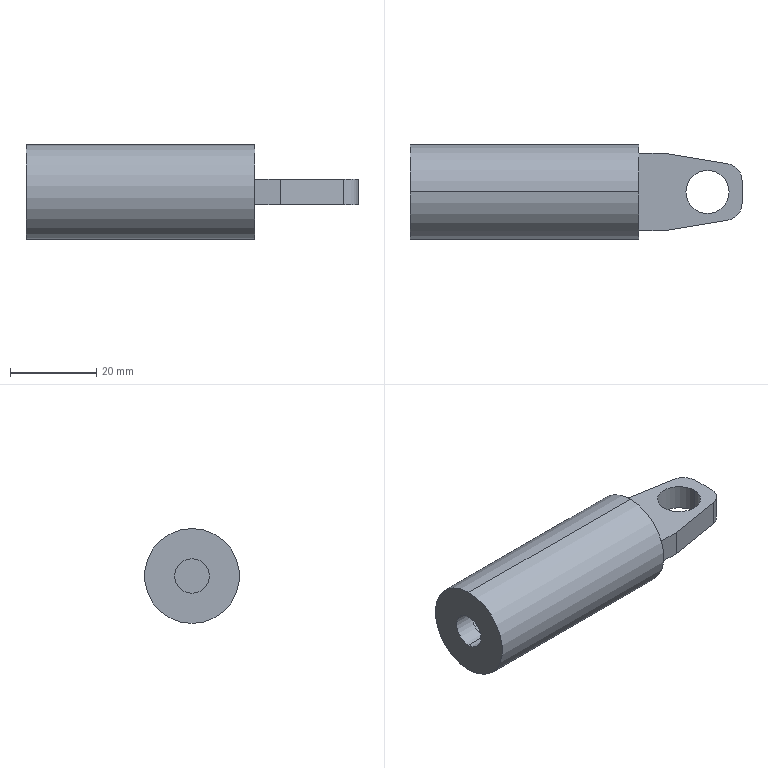Part | SolidWorks | features HoleWzd 2, Fillet 1, ICE 1, Revolution 1 | 1 solid | 21 faces | box 77 x 22 x 22 mm | volume 12617 mm3 | plane 11 | cylinder 10 | commonest cylinder face diameters 8 x4 10 x2 16 x2 22 x2
STEP:
#1=CARTESIAN_POINT('',(5.,0.,-4.));
#2=VERTEX_POINT('',#1);
#3=CARTESIAN_POINT('',(5.,0.,4.));
#4=VERTEX_POINT('',#3);
#5=CARTESIAN_POINT('',(5.,0.,0.));
#6=DIRECTION('',(-1.,0.,0.));
#7=DIRECTION('',(0.,0.,1.));
#8=AXIS2_PLACEMENT_3D('',#5,#6,#7);
#9=CIRCLE('',#8,4.);
#10=EDGE_CURVE('',#2,#4,#9,.T.);
#11=ORIENTED_EDGE('',*,*,#10,.F.);
#12=CARTESIAN_POINT('',(0.,0.,-4.));
#13=VERTEX_POINT('',#12);
#14=CARTESIAN_POINT('',(0.,0.,-4.));
#15=DIRECTION('',(-1.,0.,0.));
#16=VECTOR('',#15,1000.);
#17=LINE('',#14,#16);
#18=EDGE_CURVE('',#2,#13,#17,.T.);
#19=ORIENTED_EDGE('',*,*,#18,.T.);
#20=CARTESIAN_POINT('',(0.,0.,4.));
#21=VERTEX_POINT('',#20);
#22=CARTESIAN_POINT('',(0.,0.,0.));
#23=DIRECTION('',(-1.,0.,0.));
#24=DIRECTION('',(0.,0.,1.));
#25=AXIS2_PLACEMENT_3D('',#22,#23,#24);
#26=CIRCLE('',#25,4.);
#27=EDGE_CURVE('',#13,#21,#26,.T.);
#28=ORIENTED_EDGE('',*,*,#27,.T.);
#29=CARTESIAN_POINT('',(0.,0.,4.));
#30=DIRECTION('',(-1.,0.,0.));
#31=VECTOR('',#30,1000.);
#32=LINE('',#29,#31);
#33=EDGE_CURVE('',#4,#21,#32,.T.);
#34=ORIENTED_EDGE('',*,*,#33,.F.);
#35=EDGE_LOOP('',(#11,#19,#28,#34));
#36=FACE_OUTER_BOUND('',#35,.T.);
#37=CARTESIAN_POINT('',(0.,0.,0.));
#38=DIRECTION('',(-1.,0.,0.));
#39=DIRECTION('',(0.,0.,1.));
#40=AXIS2_PLACEMENT_3D('',#37,#38,#39);
#41=CYLINDRICAL_SURFACE('',#40,4.);
#42=ADVANCED_FACE('',(#36),#41,.F.);
#43=CARTESIAN_POINT('',(50.,0.,-8.));
#44=VERTEX_POINT('',#43);
#45=CARTESIAN_POINT('',(50.,0.,8.));
#46=VERTEX_POINT('',#45);
#47=CARTESIAN_POINT('',(50.,0.,0.));
#48=DIRECTION('',(-1.,0.,0.));
#49=DIRECTION('',(0.,0.,1.));
#50=AXIS2_PLACEMENT_3D('',#47,#48,#49);
#51=CIRCLE('',#50,8.);
#52=EDGE_CURVE('',#44,#46,#51,.T.);
#53=ORIENTED_EDGE('',*,*,#52,.F.);
#54=CARTESIAN_POINT('',(5.,0.,-8.));
#55=VERTEX_POINT('',#54);
#56=CARTESIAN_POINT('',(0.,0.,-8.));
#57=DIRECTION('',(-1.,0.,0.));
#58=VECTOR('',#57,1000.);
#59=LINE('',#56,#58);
#60=EDGE_CURVE('',#44,#55,#59,.T.);
#61=ORIENTED_EDGE('',*,*,#60,.T.);
#62=CARTESIAN_POINT('',(5.,0.,8.));
#63=VERTEX_POINT('',#62);
#64=CARTESIAN_POINT('',(5.,0.,0.));
#65=DIRECTION('',(-1.,0.,0.));
#66=DIRECTION('',(0.,0.,1.));
#67=AXIS2_PLACEMENT_3D('',#64,#65,#66);
#68=CIRCLE('',#67,8.);
#69=EDGE_CURVE('',#55,#63,#68,.T.);
#70=ORIENTED_EDGE('',*,*,#69,.T.);
#71=CARTESIAN_POINT('',(0.,0.,8.));
#72=DIRECTION('',(-1.,0.,0.));
#73=VECTOR('',#72,1000.);
#74=LINE('',#71,#73);
#75=EDGE_CURVE('',#46,#63,#74,.T.);
#76=ORIENTED_EDGE('',*,*,#75,.F.);
#77=EDGE_LOOP('',(#53,#61,#70,#76));
#78=FACE_OUTER_BOUND('',#77,.T.);
#79=CARTESIAN_POINT('',(0.,0.,0.));
#80=DIRECTION('',(-1.,0.,0.));
#81=DIRECTION('',(0.,0.,1.));
#82=AXIS2_PLACEMENT_3D('',#79,#80,#81);
#83=CYLINDRICAL_SURFACE('',#82,8.);
#84=ADVANCED_FACE('',(#78),#83,.F.);
#85=CARTESIAN_POINT('',(64.,0.,3.));
#86=VERTEX_POINT('',#85);
#87=CARTESIAN_POINT('',(74.,0.,3.));
#88=VERTEX_POINT('',#87);
#89=CARTESIAN_POINT('',(69.,0.,3.));
#90=DIRECTION('',(0.,0.,1.));
#91=DIRECTION('',(1.,0.,0.));
#92=AXIS2_PLACEMENT_3D('',#89,#90,#91);
#93=CIRCLE('',#92,5.);
#94=EDGE_CURVE('',#86,#88,#93,.T.);
#95=ORIENTED_EDGE('',*,*,#94,.T.);
#96=CARTESIAN_POINT('',(74.,0.,-3.));
#97=VERTEX_POINT('',#96);
#98=CARTESIAN_POINT('',(74.,0.,-3.));
#99=DIRECTION('',(0.,0.,-1.));
#100=VECTOR('',#99,1000.);
#101=LINE('',#98,#100);
#102=EDGE_CURVE('',#88,#97,#101,.T.);
#103=ORIENTED_EDGE('',*,*,#102,.T.);
#104=CARTESIAN_POINT('',(64.,0.,-3.));
#105=VERTEX_POINT('',#104);
#106=CARTESIAN_POINT('',(69.,0.,-3.));
#107=DIRECTION('',(0.,0.,-1.));
#108=DIRECTION('',(-1.,0.,0.));
#109=AXIS2_PLACEMENT_3D('',#106,#107,#108);
#110=CIRCLE('',#109,5.);
#111=EDGE_CURVE('',#97,#105,#110,.T.);
#112=ORIENTED_EDGE('',*,*,#111,.T.);
#113=CARTESIAN_POINT('',(64.,0.,-3.));
#114=DIRECTION('',(0.,0.,-1.));
#115=VECTOR('',#114,1000.);
#116=LINE('',#113,#115);
#117=EDGE_CURVE('',#86,#105,#116,.T.);
#118=ORIENTED_EDGE('',*,*,#117,.F.);
#119=EDGE_LOOP('',(#95,#103,#112,#118));
#120=FACE_OUTER_BOUND('',#119,.T.);
#121=CARTESIAN_POINT('',(69.,0.,-3.));
#122=DIRECTION('',(0.,0.,-1.));
#123=DIRECTION('',(-1.,0.,0.));
#124=AXIS2_PLACEMENT_3D('',#121,#122,#123);
#125=CYLINDRICAL_SURFACE('',#124,5.);
#126=ADVANCED_FACE('',(#120),#125,.F.);
#127=CARTESIAN_POINT('',(0.,0.,-11.));
#128=VERTEX_POINT('',#127);
#129=CARTESIAN_POINT('',(0.,0.,11.));
#130=VERTEX_POINT('',#129);
#131=CARTESIAN_POINT('',(0.,0.,0.));
#132=DIRECTION('',(1.,0.,0.));
#133=DIRECTION('',(0.,0.,-1.));
#134=AXIS2_PLACEMENT_3D('',#131,#132,#133);
#135=CIRCLE('',#134,11.);
#136=EDGE_CURVE('',#128,#130,#135,.T.);
#137=ORIENTED_EDGE('',*,*,#136,.T.);
#138=CARTESIAN_POINT('',(53.,0.,11.));
#139=VERTEX_POINT('',#138);
#140=CARTESIAN_POINT('',(0.,0.,11.));
#141=DIRECTION('',(1.,0.,0.));
#142=VECTOR('',#141,1000.);
#143=LINE('',#140,#142);
#144=EDGE_CURVE('',#130,#139,#143,.T.);
#145=ORIENTED_EDGE('',*,*,#144,.T.);
#146=CARTESIAN_POINT('',(53.,0.,-11.));
#147=VERTEX_POINT('',#146);
#148=CARTESIAN_POINT('',(53.,0.,0.));
#149=DIRECTION('',(1.,0.,0.));
#150=DIRECTION('',(0.,0.,-1.));
#151=AXIS2_PLACEMENT_3D('',#148,#149,#150);
#152=CIRCLE('',#151,11.);
#153=EDGE_CURVE('',#147,#139,#152,.T.);
#154=ORIENTED_EDGE('',*,*,#153,.F.);
#155=CARTESIAN_POINT('',(0.,0.,-11.));
#156=DIRECTION('',(1.,0.,0.));
#157=VECTOR('',#156,1000.);
#158=LINE('',#155,#157);
#159=EDGE_CURVE('',#128,#147,#158,.T.);
#160=ORIENTED_EDGE('',*,*,#159,.F.);
#161=EDGE_LOOP('',(#137,#145,#154,#160));
#162=FACE_OUTER_BOUND('',#161,.T.);
#163=CARTESIAN_POINT('',(0.,0.,0.));
#164=DIRECTION('',(1.,0.,0.));
#165=DIRECTION('',(0.,0.,-1.));
#166=AXIS2_PLACEMENT_3D('',#163,#164,#165);
#167=CYLINDRICAL_SURFACE('',#166,11.);
#168=ADVANCED_FACE('',(#162),#167,.T.);
#169=ORIENTED_EDGE('',*,*,#144,.F.);
#170=CARTESIAN_POINT('',(0.,0.,0.));
#171=DIRECTION('',(1.,0.,0.));
#172=DIRECTION('',(0.,0.,-1.));
#173=AXIS2_PLACEMENT_3D('',#170,#171,#172);
#174=CIRCLE('',#173,11.);
#175=EDGE_CURVE('',#130,#128,#174,.T.);
#176=ORIENTED_EDGE('',*,*,#175,.T.);
#177=ORIENTED_EDGE('',*,*,#159,.T.);
#178=CARTESIAN_POINT('',(53.,0.,0.));
#179=DIRECTION('',(1.,0.,0.));
#180=DIRECTION('',(0.,0.,-1.));
#181=AXIS2_PLACEMENT_3D('',#178,#179,#180);
#182=CIRCLE('',#181,11.);
#183=EDGE_CURVE('',#139,#147,#182,.T.);
#184=ORIENTED_EDGE('',*,*,#183,.F.);
#185=EDGE_LOOP('',(#169,#176,#177,#184));
#186=FACE_OUTER_BOUND('',#185,.T.);
#187=CARTESIAN_POINT('',(0.,0.,0.));
#188=DIRECTION('',(1.,0.,0.));
#189=DIRECTION('',(0.,0.,-1.));
#190=AXIS2_PLACEMENT_3D('',#187,#188,#189);
#191=CYLINDRICAL_SURFACE('',#190,11.);
#192=ADVANCED_FACE('',(#186),#191,.T.);
#193=CARTESIAN_POINT('',(0.,0.,0.));
#194=DIRECTION('',(-1.,0.,0.));
#195=DIRECTION('',(0.,0.,1.));
#196=AXIS2_PLACEMENT_3D('',#193,#194,#195);
#197=CIRCLE('',#196,4.);
#198=EDGE_CURVE('',#21,#13,#197,.T.);
#199=ORIENTED_EDGE('',*,*,#198,.F.);
#200=ORIENTED_EDGE('',*,*,#27,.F.);
#201=EDGE_LOOP('',(#199,#200));
#202=FACE_BOUND('',#201,.T.);
#203=ORIENTED_EDGE('',*,*,#136,.F.);
#204=ORIENTED_EDGE('',*,*,#175,.F.);
#205=EDGE_LOOP('',(#203,#204));
#206=FACE_OUTER_BOUND('',#205,.T.);
#207=CARTESIAN_POINT('',(0.,11.,0.));
#208=DIRECTION('',(-1.,0.,0.));
#209=DIRECTION('',(0.,0.,1.));
#210=AXIS2_PLACEMENT_3D('',#207,#208,#209);
#211=PLANE('',#210);
#212=ADVANCED_FACE('',(#202,#206),#211,.T.);
#213=CARTESIAN_POINT('',(53.,9.,3.));
#214=VERTEX_POINT('',#213);
#215=CARTESIAN_POINT('',(53.,-9.,3.));
#216=VERTEX_POINT('',#215);
#217=CARTESIAN_POINT('',(53.,9.,3.));
#218=DIRECTION('',(0.,-1.,0.));
#219=VECTOR('',#218,1000.);
#220=LINE('',#217,#219);
#221=EDGE_CURVE('',#214,#216,#220,.T.);
#222=ORIENTED_EDGE('',*,*,#221,.F.);
#223=CARTESIAN_POINT('',(53.,9.,-3.));
#224=VERTEX_POINT('',#223);
#225=CARTESIAN_POINT('',(53.,9.,-3.));
#226=DIRECTION('',(0.,0.,1.));
#227=VECTOR('',#226,1000.);
#228=LINE('',#225,#227);
#229=EDGE_CURVE('',#224,#214,#228,.T.);
#230=ORIENTED_EDGE('',*,*,#229,.F.);
#231=CARTESIAN_POINT('',(53.,-9.,-3.));
#232=VERTEX_POINT('',#231);
#233=CARTESIAN_POINT('',(53.,9.,-3.));
#234=DIRECTION('',(0.,-1.,0.));
#235=VECTOR('',#234,1000.);
#236=LINE('',#233,#235);
#237=EDGE_CURVE('',#224,#232,#236,.T.);
#238=ORIENTED_EDGE('',*,*,#237,.T.);
#239=CARTESIAN_POINT('',(53.,-9.,-3.));
#240=DIRECTION('',(0.,0.,1.));
#241=VECTOR('',#240,1000.);
#242=LINE('',#239,#241);
#243=EDGE_CURVE('',#232,#216,#242,.T.);
#244=ORIENTED_EDGE('',*,*,#243,.T.);
#245=EDGE_LOOP('',(#222,#230,#238,#244));
#246=FACE_BOUND('',#245,.T.);
#247=ORIENTED_EDGE('',*,*,#153,.T.);
#248=ORIENTED_EDGE('',*,*,#183,.T.);
#249=EDGE_LOOP('',(#247,#248));
#250=FACE_OUTER_BOUND('',#249,.T.);
#251=CARTESIAN_POINT('',(53.,0.,0.));
#252=DIRECTION('',(1.,0.,0.));
#253=DIRECTION('',(0.,0.,-1.));
#254=AXIS2_PLACEMENT_3D('',#251,#252,#253);
#255=PLANE('',#254);
#256=ADVANCED_FACE('',(#246,#250),#255,.T.);
#257=CARTESIAN_POINT('',(59.,-9.,-3.));
#258=VERTEX_POINT('',#257);
#259=CARTESIAN_POINT('',(73.658,-6.557,-3.));
#260=VERTEX_POINT('',#259);
#261=CARTESIAN_POINT('',(59.,-9.,-3.));
#262=DIRECTION('',(0.9864,0.1644,0.));
#263=VECTOR('',#262,1000.);
#264=LINE('',#261,#263);
#265=EDGE_CURVE('',#258,#260,#264,.T.);
#266=ORIENTED_EDGE('',*,*,#265,.T.);
#267=CARTESIAN_POINT('',(73.658,-6.557,3.));
#268=VERTEX_POINT('',#267);
#269=CARTESIAN_POINT('',(73.658,-6.557,-3.));
#270=DIRECTION('',(0.,0.,1.));
#271=VECTOR('',#270,1000.);
#272=LINE('',#269,#271);
#273=EDGE_CURVE('',#260,#268,#272,.T.);
#274=ORIENTED_EDGE('',*,*,#273,.T.);
#275=CARTESIAN_POINT('',(59.,-9.,3.));
#276=VERTEX_POINT('',#275);
#277=CARTESIAN_POINT('',(59.,-9.,3.));
#278=DIRECTION('',(0.9864,0.1644,0.));
#279=VECTOR('',#278,1000.);
#280=LINE('',#277,#279);
#281=EDGE_CURVE('',#276,#268,#280,.T.);
#282=ORIENTED_EDGE('',*,*,#281,.F.);
#283=CARTESIAN_POINT('',(59.,-9.,-3.));
#284=DIRECTION('',(0.,0.,1.));
#285=VECTOR('',#284,1000.);
#286=LINE('',#283,#285);
#287=EDGE_CURVE('',#258,#276,#286,.T.);
#288=ORIENTED_EDGE('',*,*,#287,.F.);
#289=EDGE_LOOP('',(#266,#274,#282,#288));
#290=FACE_OUTER_BOUND('',#289,.T.);
#291=CARTESIAN_POINT('',(59.,-9.,-3.));
#292=DIRECTION('',(0.1644,-0.9864,0.));
#293=DIRECTION('',(0.9864,0.1644,0.));
#294=AXIS2_PLACEMENT_3D('',#291,#292,#293);
#295=PLANE('',#294);
#296=ADVANCED_FACE('',(#290),#295,.T.);
#297=CARTESIAN_POINT('',(53.,-9.,3.));
#298=DIRECTION('',(1.,0.,0.));
#299=VECTOR('',#298,1000.);
#300=LINE('',#297,#299);
#301=EDGE_CURVE('',#216,#276,#300,.T.);
#302=ORIENTED_EDGE('',*,*,#301,.F.);
#303=ORIENTED_EDGE('',*,*,#243,.F.);
#304=CARTESIAN_POINT('',(53.,-9.,-3.));
#305=DIRECTION('',(1.,0.,0.));
#306=VECTOR('',#305,1000.);
#307=LINE('',#304,#306);
#308=EDGE_CURVE('',#232,#258,#307,.T.);
#309=ORIENTED_EDGE('',*,*,#308,.T.);
#310=ORIENTED_EDGE('',*,*,#287,.T.);
#311=EDGE_LOOP('',(#302,#303,#309,#310));
#312=FACE_OUTER_BOUND('',#311,.T.);
#313=CARTESIAN_POINT('',(53.,-9.,-3.));
#314=DIRECTION('',(0.,-1.,0.));
#315=DIRECTION('',(0.,0.,-1.));
#316=AXIS2_PLACEMENT_3D('',#313,#314,#315);
#317=PLANE('',#316);
#318=ADVANCED_FACE('',(#312),#317,.T.);
#319=CARTESIAN_POINT('',(59.,9.,3.));
#320=VERTEX_POINT('',#319);
#321=CARTESIAN_POINT('',(59.,9.,3.));
#322=DIRECTION('',(-1.,0.,0.));
#323=VECTOR('',#322,1000.);
#324=LINE('',#321,#323);
#325=EDGE_CURVE('',#320,#214,#324,.T.);
#326=ORIENTED_EDGE('',*,*,#325,.F.);
#327=CARTESIAN_POINT('',(59.,9.,-3.));
#328=VERTEX_POINT('',#327);
#329=CARTESIAN_POINT('',(59.,9.,-3.));
#330=DIRECTION('',(0.,0.,1.));
#331=VECTOR('',#330,1000.);
#332=LINE('',#329,#331);
#333=EDGE_CURVE('',#328,#320,#332,.T.);
#334=ORIENTED_EDGE('',*,*,#333,.F.);
#335=CARTESIAN_POINT('',(59.,9.,-3.));
#336=DIRECTION('',(-1.,0.,0.));
#337=VECTOR('',#336,1000.);
#338=LINE('',#335,#337);
#339=EDGE_CURVE('',#328,#224,#338,.T.);
#340=ORIENTED_EDGE('',*,*,#339,.T.);
#341=ORIENTED_EDGE('',*,*,#229,.T.);
#342=EDGE_LOOP('',(#326,#334,#340,#341));
#343=FACE_OUTER_BOUND('',#342,.T.);
#344=CARTESIAN_POINT('',(59.,9.,-3.));
#345=DIRECTION('',(0.,1.,0.));
#346=DIRECTION('',(0.,0.,1.));
#347=AXIS2_PLACEMENT_3D('',#344,#345,#346);
#348=PLANE('',#347);
#349=ADVANCED_FACE('',(#343),#348,.T.);
#350=CARTESIAN_POINT('',(73.658,6.557,3.));
#351=VERTEX_POINT('',#350);
#352=CARTESIAN_POINT('',(77.,6.,3.));
#353=DIRECTION('',(-0.9864,0.1644,0.));
#354=VECTOR('',#353,1000.);
#355=LINE('',#352,#354);
#356=EDGE_CURVE('',#351,#320,#355,.T.);
#357=ORIENTED_EDGE('',*,*,#356,.F.);
#358=CARTESIAN_POINT('',(73.658,6.557,-3.));
#359=VERTEX_POINT('',#358);
#360=CARTESIAN_POINT('',(73.658,6.557,-3.));
#361=DIRECTION('',(0.,0.,-1.));
#362=VECTOR('',#361,1000.);
#363=LINE('',#360,#362);
#364=EDGE_CURVE('',#351,#359,#363,.T.);
#365=ORIENTED_EDGE('',*,*,#364,.T.);
#366=CARTESIAN_POINT('',(77.,6.,-3.));
#367=DIRECTION('',(-0.9864,0.1644,0.));
#368=VECTOR('',#367,1000.);
#369=LINE('',#366,#368);
#370=EDGE_CURVE('',#359,#328,#369,.T.);
#371=ORIENTED_EDGE('',*,*,#370,.T.);
#372=ORIENTED_EDGE('',*,*,#333,.T.);
#373=EDGE_LOOP('',(#357,#365,#371,#372));
#374=FACE_OUTER_BOUND('',#373,.T.);
#375=CARTESIAN_POINT('',(77.,6.,-3.));
#376=DIRECTION('',(0.1644,0.9864,0.));
#377=DIRECTION('',(-0.9864,0.1644,0.));
#378=AXIS2_PLACEMENT_3D('',#375,#376,#377);
#379=PLANE('',#378);
#380=ADVANCED_FACE('',(#374),#379,.T.);
#381=CARTESIAN_POINT('',(77.,-2.611,-3.));
#382=VERTEX_POINT('',#381);
#383=CARTESIAN_POINT('',(77.,2.611,-3.));
#384=VERTEX_POINT('',#383);
#385=CARTESIAN_POINT('',(77.,-6.,-3.));
#386=DIRECTION('',(0.,1.,0.));
#387=VECTOR('',#386,1000.);
#388=LINE('',#385,#387);
#389=EDGE_CURVE('',#382,#384,#388,.T.);
#390=ORIENTED_EDGE('',*,*,#389,.T.);
#391=CARTESIAN_POINT('',(77.,2.611,3.));
#392=VERTEX_POINT('',#391);
#393=CARTESIAN_POINT('',(77.,2.611,-3.));
#394=DIRECTION('',(0.,0.,1.));
#395=VECTOR('',#394,1000.);
#396=LINE('',#393,#395);
#397=EDGE_CURVE('',#384,#392,#396,.T.);
#398=ORIENTED_EDGE('',*,*,#397,.T.);
#399=CARTESIAN_POINT('',(77.,-2.611,3.));
#400=VERTEX_POINT('',#399);
#401=CARTESIAN_POINT('',(77.,-6.,3.));
#402=DIRECTION('',(0.,1.,0.));
#403=VECTOR('',#402,1000.);
#404=LINE('',#401,#403);
#405=EDGE_CURVE('',#400,#392,#404,.T.);
#406=ORIENTED_EDGE('',*,*,#405,.F.);
#407=CARTESIAN_POINT('',(77.,-2.611,-3.));
#408=DIRECTION('',(0.,0.,-1.));
#409=VECTOR('',#408,1000.);
#410=LINE('',#407,#409);
#411=EDGE_CURVE('',#400,#382,#410,.T.);
#412=ORIENTED_EDGE('',*,*,#411,.T.);
#413=EDGE_LOOP('',(#390,#398,#406,#412));
#414=FACE_OUTER_BOUND('',#413,.T.);
#415=CARTESIAN_POINT('',(77.,-6.,-3.));
#416=DIRECTION('',(1.,0.,0.));
#417=DIRECTION('',(0.,0.,-1.));
#418=AXIS2_PLACEMENT_3D('',#415,#416,#417);
#419=PLANE('',#418);
#420=ADVANCED_FACE('',(#414),#419,.T.);
#421=CARTESIAN_POINT('',(69.,0.,-3.));
#422=DIRECTION('',(0.,0.,-1.));
#423=DIRECTION('',(-1.,0.,0.));
#424=AXIS2_PLACEMENT_3D('',#421,#422,#423);
#425=CIRCLE('',#424,5.);
#426=EDGE_CURVE('',#105,#97,#425,.T.);
#427=ORIENTED_EDGE('',*,*,#426,.F.);
#428=ORIENTED_EDGE('',*,*,#111,.F.);
#429=EDGE_LOOP('',(#427,#428));
#430=FACE_BOUND('',#429,.T.);
#431=ORIENTED_EDGE('',*,*,#370,.F.);
#432=CARTESIAN_POINT('',(73.,2.611,-3.));
#433=DIRECTION('',(0.,0.,-1.));
#434=DIRECTION('',(1.,0.,0.));
#435=AXIS2_PLACEMENT_3D('',#432,#433,#434);
#436=CIRCLE('',#435,4.);
#437=EDGE_CURVE('',#359,#384,#436,.T.);
#438=ORIENTED_EDGE('',*,*,#437,.T.);
#439=ORIENTED_EDGE('',*,*,#389,.F.);
#440=CARTESIAN_POINT('',(73.,-2.611,-3.));
#441=DIRECTION('',(0.,0.,-1.));
#442=DIRECTION('',(1.,0.,0.));
#443=AXIS2_PLACEMENT_3D('',#440,#441,#442);
#444=CIRCLE('',#443,4.);
#445=EDGE_CURVE('',#382,#260,#444,.T.);
#446=ORIENTED_EDGE('',*,*,#445,.T.);
#447=ORIENTED_EDGE('',*,*,#265,.F.);
#448=ORIENTED_EDGE('',*,*,#308,.F.);
#449=ORIENTED_EDGE('',*,*,#237,.F.);
#450=ORIENTED_EDGE('',*,*,#339,.F.);
#451=EDGE_LOOP('',(#431,#438,#439,#446,#447,#448,#449,#450));
#452=FACE_OUTER_BOUND('',#451,.T.);
#453=CARTESIAN_POINT('',(0.,0.,-3.));
#454=DIRECTION('',(0.,0.,1.));
#455=DIRECTION('',(1.,0.,0.));
#456=AXIS2_PLACEMENT_3D('',#453,#454,#455);
#457=PLANE('',#456);
#458=ADVANCED_FACE('',(#430,#452),#457,.F.);
#459=ORIENTED_EDGE('',*,*,#94,.F.);
#460=CARTESIAN_POINT('',(69.,0.,3.));
#461=DIRECTION('',(0.,0.,1.));
#462=DIRECTION('',(1.,0.,0.));
#463=AXIS2_PLACEMENT_3D('',#460,#461,#462);
#464=CIRCLE('',#463,5.);
#465=EDGE_CURVE('',#88,#86,#464,.T.);
#466=ORIENTED_EDGE('',*,*,#465,.F.);
#467=EDGE_LOOP('',(#459,#466));
#468=FACE_BOUND('',#467,.T.);
#469=ORIENTED_EDGE('',*,*,#405,.T.);
#470=CARTESIAN_POINT('',(73.,2.611,3.));
#471=DIRECTION('',(0.,0.,1.));
#472=DIRECTION('',(1.,0.,0.));
#473=AXIS2_PLACEMENT_3D('',#470,#471,#472);
#474=CIRCLE('',#473,4.);
#475=EDGE_CURVE('',#392,#351,#474,.T.);
#476=ORIENTED_EDGE('',*,*,#475,.T.);
#477=ORIENTED_EDGE('',*,*,#356,.T.);
#478=ORIENTED_EDGE('',*,*,#325,.T.);
#479=ORIENTED_EDGE('',*,*,#221,.T.);
#480=ORIENTED_EDGE('',*,*,#301,.T.);
#481=ORIENTED_EDGE('',*,*,#281,.T.);
#482=CARTESIAN_POINT('',(73.,-2.611,3.));
#483=DIRECTION('',(0.,0.,1.));
#484=DIRECTION('',(1.,0.,0.));
#485=AXIS2_PLACEMENT_3D('',#482,#483,#484);
#486=CIRCLE('',#485,4.);
#487=EDGE_CURVE('',#268,#400,#486,.T.);
#488=ORIENTED_EDGE('',*,*,#487,.T.);
#489=EDGE_LOOP('',(#469,#476,#477,#478,#479,#480,#481,#488));
#490=FACE_OUTER_BOUND('',#489,.T.);
#491=CARTESIAN_POINT('',(0.,0.,3.));
#492=DIRECTION('',(0.,0.,1.));
#493=DIRECTION('',(1.,0.,0.));
#494=AXIS2_PLACEMENT_3D('',#491,#492,#493);
#495=PLANE('',#494);
#496=ADVANCED_FACE('',(#468,#490),#495,.T.);
#497=ORIENTED_EDGE('',*,*,#102,.F.);
#498=ORIENTED_EDGE('',*,*,#465,.T.);
#499=ORIENTED_EDGE('',*,*,#117,.T.);
#500=ORIENTED_EDGE('',*,*,#426,.T.);
#501=EDGE_LOOP('',(#497,#498,#499,#500));
#502=FACE_OUTER_BOUND('',#501,.T.);
#503=CARTESIAN_POINT('',(69.,0.,-3.));
#504=DIRECTION('',(0.,0.,-1.));
#505=DIRECTION('',(-1.,0.,0.));
#506=AXIS2_PLACEMENT_3D('',#503,#504,#505);
#507=CYLINDRICAL_SURFACE('',#506,5.);
#508=ADVANCED_FACE('',(#502),#507,.F.);
#509=CARTESIAN_POINT('',(50.,0.,0.));
#510=DIRECTION('',(-1.,0.,0.));
#511=DIRECTION('',(0.,0.,1.));
#512=AXIS2_PLACEMENT_3D('',#509,#510,#511);
#513=CIRCLE('',#512,8.);
#514=EDGE_CURVE('',#46,#44,#513,.T.);
#515=ORIENTED_EDGE('',*,*,#514,.T.);
#516=ORIENTED_EDGE('',*,*,#52,.T.);
#517=EDGE_LOOP('',(#515,#516));
#518=FACE_OUTER_BOUND('',#517,.T.);
#519=CARTESIAN_POINT('',(50.,0.,0.));
#520=DIRECTION('',(1.,0.,0.));
#521=DIRECTION('',(0.,0.,-1.));
#522=AXIS2_PLACEMENT_3D('',#519,#520,#521);
#523=PLANE('',#522);
#524=ADVANCED_FACE('',(#518),#523,.F.);
#525=ORIENTED_EDGE('',*,*,#60,.F.);
#526=ORIENTED_EDGE('',*,*,#514,.F.);
#527=ORIENTED_EDGE('',*,*,#75,.T.);
#528=CARTESIAN_POINT('',(5.,0.,0.));
#529=DIRECTION('',(-1.,0.,0.));
#530=DIRECTION('',(0.,0.,1.));
#531=AXIS2_PLACEMENT_3D('',#528,#529,#530);
#532=CIRCLE('',#531,8.);
#533=EDGE_CURVE('',#63,#55,#532,.T.);
#534=ORIENTED_EDGE('',*,*,#533,.T.);
#535=EDGE_LOOP('',(#525,#526,#527,#534));
#536=FACE_OUTER_BOUND('',#535,.T.);
#537=CARTESIAN_POINT('',(0.,0.,0.));
#538=DIRECTION('',(-1.,0.,0.));
#539=DIRECTION('',(0.,0.,1.));
#540=AXIS2_PLACEMENT_3D('',#537,#538,#539);
#541=CYLINDRICAL_SURFACE('',#540,8.);
#542=ADVANCED_FACE('',(#536),#541,.F.);
#543=ORIENTED_EDGE('',*,*,#533,.F.);
#544=ORIENTED_EDGE('',*,*,#69,.F.);
#545=EDGE_LOOP('',(#543,#544));
#546=FACE_OUTER_BOUND('',#545,.T.);
#547=CARTESIAN_POINT('',(5.,0.,0.));
#548=DIRECTION('',(-1.,0.,0.));
#549=DIRECTION('',(0.,0.,1.));
#550=AXIS2_PLACEMENT_3D('',#547,#548,#549);
#551=CIRCLE('',#550,4.);
#552=EDGE_CURVE('',#4,#2,#551,.T.);
#553=ORIENTED_EDGE('',*,*,#552,.T.);
#554=ORIENTED_EDGE('',*,*,#10,.T.);
#555=EDGE_LOOP('',(#553,#554));
#556=FACE_BOUND('',#555,.T.);
#557=CARTESIAN_POINT('',(5.,8.,0.));
#558=DIRECTION('',(-1.,0.,0.));
#559=DIRECTION('',(0.,0.,1.));
#560=AXIS2_PLACEMENT_3D('',#557,#558,#559);
#561=PLANE('',#560);
#562=ADVANCED_FACE('',(#546,#556),#561,.F.);
#563=ORIENTED_EDGE('',*,*,#18,.F.);
#564=ORIENTED_EDGE('',*,*,#552,.F.);
#565=ORIENTED_EDGE('',*,*,#33,.T.);
#566=ORIENTED_EDGE('',*,*,#198,.T.);
#567=EDGE_LOOP('',(#563,#564,#565,#566));
#568=FACE_OUTER_BOUND('',#567,.T.);
#569=CARTESIAN_POINT('',(0.,0.,0.));
#570=DIRECTION('',(-1.,0.,0.));
#571=DIRECTION('',(0.,0.,1.));
#572=AXIS2_PLACEMENT_3D('',#569,#570,#571);
#573=CYLINDRICAL_SURFACE('',#572,4.);
#574=ADVANCED_FACE('',(#568),#573,.F.);
#575=ORIENTED_EDGE('',*,*,#437,.F.);
#576=ORIENTED_EDGE('',*,*,#364,.F.);
#577=ORIENTED_EDGE('',*,*,#475,.F.);
#578=ORIENTED_EDGE('',*,*,#397,.F.);
#579=EDGE_LOOP('',(#575,#576,#577,#578));
#580=FACE_OUTER_BOUND('',#579,.T.);
#581=CARTESIAN_POINT('',(73.,2.611,-3.));
#582=DIRECTION('',(0.,0.,1.));
#583=DIRECTION('',(1.,0.,0.));
#584=AXIS2_PLACEMENT_3D('',#581,#582,#583);
#585=CYLINDRICAL_SURFACE('',#584,4.);
#586=ADVANCED_FACE('',(#580),#585,.T.);
#587=ORIENTED_EDGE('',*,*,#445,.F.);
#588=ORIENTED_EDGE('',*,*,#411,.F.);
#589=ORIENTED_EDGE('',*,*,#487,.F.);
#590=ORIENTED_EDGE('',*,*,#273,.F.);
#591=EDGE_LOOP('',(#587,#588,#589,#590));
#592=FACE_OUTER_BOUND('',#591,.T.);
#593=CARTESIAN_POINT('',(73.,-2.611,-3.));
#594=DIRECTION('',(0.,0.,1.));
#595=DIRECTION('',(1.,0.,0.));
#596=AXIS2_PLACEMENT_3D('',#593,#594,#595);
#597=CYLINDRICAL_SURFACE('',#596,4.);
#598=ADVANCED_FACE('',(#592),#597,.T.);
#599=CLOSED_SHELL('',(#42,#84,#126,#168,#192,#212,#256,#296,#318,#349,#380,#420,#458,#496,#508,#524,#542,#562,#574,#586,#598));
#600=MANIFOLD_SOLID_BREP('',#599);
#601=CARTESIAN_POINT('',(0.,0.,0.));
#602=DIRECTION('',(0.,0.,1.));
#603=DIRECTION('',(1.,0.,0.));
#604=AXIS2_PLACEMENT_3D('',#601,#602,#603);
#605=(LENGTH_UNIT()NAMED_UNIT(*)SI_UNIT(.MILLI.,.METRE.));
#606=UNCERTAINTY_MEASURE_WITH_UNIT(LENGTH_MEASURE(0.00001),#605,'','');
#607=(NAMED_UNIT(*)PLANE_ANGLE_UNIT()SI_UNIT($,.RADIAN.));
#608=(NAMED_UNIT(*)SI_UNIT($,.STERADIAN.)SOLID_ANGLE_UNIT());
#609=(GEOMETRIC_REPRESENTATION_CONTEXT(3)GLOBAL_UNCERTAINTY_ASSIGNED_CONTEXT((#606))GLOBAL_UNIT_ASSIGNED_CONTEXT((#605,#607,#608))REPRESENTATION_CONTEXT('',''));
#610=ADVANCED_BREP_SHAPE_REPRESENTATION('',(#600,#604),#609);